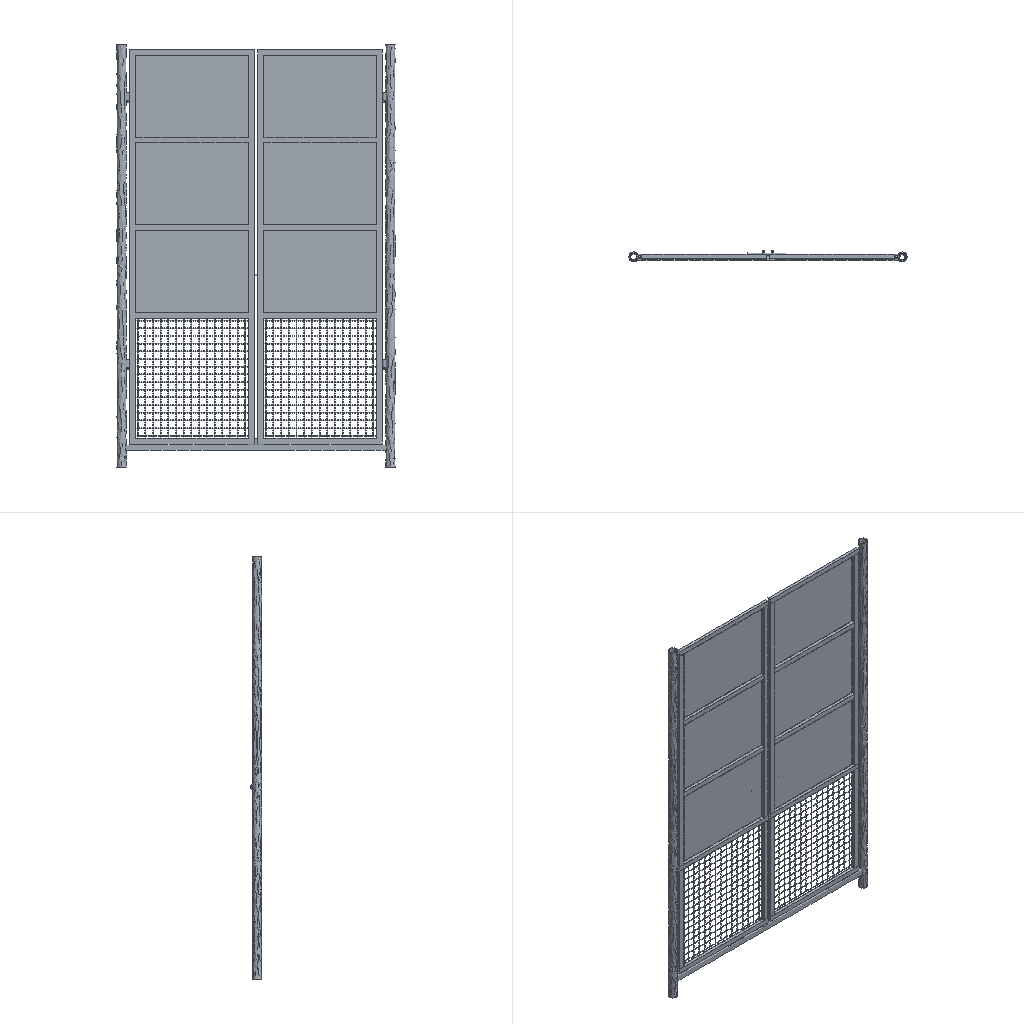Simulation study | ansys workbench
Set-up summary:
category,name,step,type,value,unit,region
solver,ansys_mapdl
solver,version,,,25.2
solver,version,,,25.2
solver,version,,,25.2
solver,version,,,25.2
solver,version,,,25.2
units,MKS,,stated
analysis,deck,,static,static
load_step,requested,,,1
analysis,nlgeom,,,True
mesh,nodes,,,121122
mesh,elements,,,99947
element_type,ANSYS 187 (type 1),,solid,19822
element_type,ANSYS 186 (type 2),,solid,561
element_type,ANSYS 187 (type 3),,solid,19785
element_type,ANSYS 187 (type 4),,solid,10615
element_type,ANSYS 174 (type 5),,contact,5385
element_type,ANSYS 170 (type 6),,target,5385
element_type,ANSYS 174 (type 7),,contact,6752
element_type,ANSYS 170 (type 8),,target,6752
element_type,ANSYS 174 (type 9),,contact,5458
element_type,ANSYS 170 (type 10),,target,5458
element_type,ANSYS 174 (type 11),,contact,6942
element_type,ANSYS 170 (type 12),,target,6942
element_type,ANSYS 154 (type 13),,surface,90
load,load commands in deck,,count,3
bc,support commands in deck,,count,1
named_set,_FIXEDSU,,component
material,1,,in results
material,2,,in results
material,3,,in results
material,1,,in results
material,3,,in results
material,1,,in results
material,1,,in results
material,4,,in results
material,1,,in results
material,2,,in results
material,3,,in results
material,4,,in results
check,setup vs results,,match,24537 contact/target element(s) of the setup are not in the results: solve.out records that the solver deleted 24537 by its trimming logic; 90 surface effect element(s) are not in the reader's mesh and were not compared
Ansys APDL input file, long lists of numbers shortened:
/batch
/config,noeldb,1     ! force off writing results to database
*get,_wallstrt,active,,time,wall
! ANSYS input file written by Workbench version 2025 R2
! File used for geometry attach: D:\å±é¨\fangan1\æ¹æ¡1_files\dp0\SYS\DM\SYS.dsco
/title,__1--____ (A5)
! ****** Begin Custom Load Command Snippet ******
/COM, ACT Extensions:
/COM,     LSDYNA, 2025.2
/COM,/COM,     ANSYSMotion, 2025.2
/COM,
! ****** End   Custom Load Command Snippet ******
/com,--- Data in consistent MKS units. See Solving Units in the help system for more information.
/units,MKS
/nopr
/wb,file,start              !  signify a WB generated input file
/prep7
! Turn off shape checking because checks already performed inside WB mesher.
! See help system for more information.
SHPP,OFF,,NOWARN
/nolist
etcon,set             ! allow ANSYS to choose best KEYOP's for 180x elements, resets any applicable keyopt to MAPDL defaults
/com,*********** Send User Defined Coordinate System(s) ***********
csys,0
/com,*********** Nodes for the whole assembly ***********
nblock,3,,133234
(1i9,3e20.9e3)
    48322     1.737721569E+00     1.701438756E-02    -1.199439081E+00
! (121121 more lines like these left out)
-1
/wb,elem,start            !  set before creation of elements
/com,*********** Elements for Body 1 'SYS\__' ***********
et,1,187
MAT,1 $ TYPE,1 $ REAL,1 $ SECNUM,1 $ ESYS,0
eblock,11,COMPACT,,19822
(11i9)
        1        1     8739     8742     8896     9317    47651     9318     9319    47655    47673
! (19821 more lines like these left out)
-1
secnum,1    ! reset the section ID to default
/com,*********** Elements for Body 2 'SYS\__' ***********
et,2,186
keyo,2,2,1          ! set full integration on SOLID186
MAT,2 $ TYPE,2 $ REAL,2 $ SECNUM,2 $ ESYS,0
eblock,11,COMPACT,,561
(11i9)
    19823    48322    48325    48329    48328    48729    48726    48722    48723    49155    49168
! (1121 more lines like these left out)
-1
secnum,1    ! reset the section ID to default
/com,*********** Elements for Body 3 'SYS\__' ***********
et,3,187
MAT,3 $ TYPE,3 $ REAL,3 $ SECNUM,3 $ ESYS,0
eblock,11,COMPACT,,19785
(11i9)
    20384    53935    60208    60034    53939    79578    98792    79576    79574    79599    79598
! (19784 more lines like these left out)
-1
secnum,1    ! reset the section ID to default
/com,*********** Elements for Body 4 'SYS\__' ***********
et,4,187
MAT,4 $ TYPE,4 $ REAL,4 $ SECNUM,4 $ ESYS,0
eblock,11,COMPACT,,10615
(11i9)
    40169    99585    99920    99586    99845   103304   103312   103298   103302   104804   103311
! (10614 more lines like these left out)
-1
secnum,1    ! reset the section ID to default
/wb,elem,end               !  done creating elements
toffst,273.15,      ! Temperature offset from absolute zero
/com,*********** Set Reference Temperature ***********
tref,22.
/wb,mat,start              !  starting to send materials
/com,*********** Send Materials ***********
Temperature = 'TEMP' ! Temperature
MP,DENS,1,7850,	! kg m^-3
MP,ALPX,1,1.2e-05,	! C^-1
MP,C,1,434,	! J kg^-1 C^-1
MP,KXX,1,60.5,	! W m^-1 C^-1
MP,RSVX,1,1.7e-07,	! kg m^3 A^-2 s^-3
MP,EX,1,200000000000,	! Pa
MP,NUXY,1,0.3,
MP,MURX,1,10000,
Temperature = 'TEMP' ! Temperature
MP,DENS,2,7850,	! kg m^-3
MP,ALPX,2,1.2e-05,	! C^-1
MP,C,2,434,	! J kg^-1 C^-1
MP,KXX,2,60.5,	! W m^-1 C^-1
MP,RSVX,2,1.7e-07,	! kg m^3 A^-2 s^-3
MP,EX,2,200000000000,	! Pa
MP,NUXY,2,0.3,
MP,MURX,2,10000,
Temperature = 'TEMP' ! Temperature
MP,DENS,3,7850,	! kg m^-3
MP,ALPX,3,1.2e-05,	! C^-1
MP,C,3,434,	! J kg^-1 C^-1
MP,KXX,3,60.5,	! W m^-1 C^-1
MP,RSVX,3,1.7e-07,	! kg m^3 A^-2 s^-3
MP,EX,3,200000000000,	! Pa
MP,NUXY,3,0.3,
MP,MURX,3,10000,
Temperature = 'TEMP' ! Temperature
MP,DENS,4,7850,	! kg m^-3
MP,ALPX,4,1.2e-05,	! C^-1
MP,C,4,434,	! J kg^-1 C^-1
MP,KXX,4,60.5,	! W m^-1 C^-1
MP,RSVX,4,1.7e-07,	! kg m^3 A^-2 s^-3
MP,EX,4,200000000000,	! Pa
MP,NUXY,4,0.3,
MP,MURX,4,10000,
/wb,mat,end                !  done sending materials
!************************* Model Summary ********************
!SYS\å®ä½,	ç»æé¢,	matid,	1
!SYS\å®ä½,	ç»æé¢,	matid,	2
!SYS\å®ä½,	ç»æé¢,	matid,	3
!SYS\å®ä½,	ç»æé¢,	matid,	4
!************************* End Model Summary ********************
! get the diagonal of the bounding box. Needed later for other things
*get,_xmin,node,,mnloc,x
*get,_ymin,node,,mnloc,y
*get,_zmin,node,,mnloc,z
*get,_xmax,node,,mxloc,x
*get,_ymax,node,,mxloc,y
*get,_zmax,node,,mxloc,z
_ASMDIAG=(_xmax-_xmin)*(_xmax-_xmin)+(_ymax-_ymin)*(_ymax-_ymin)+(_zmax-_zmin)*(_zmax-_zmin)
_ASMDIAG=SQRT(_ASMDIAG)
/wb,contact,start          !  starting to send contact
/com,*********** Create Contact "ÎÞÄ¦²Á - SYS\ÊµÌå Î»ÓÚ SYS\ÊµÌå" ***********
/com,            Real Constant Set For Above Contact Is 6 & 5
*set,tid,6
*set,cid,5
r,tid
r,cid
et,tid,170
et,cid,174
MAT,6 $ TYPE,6 $ REAL,6 $ SECNUM,6 $ ESYS,0
eblock,11,COMPACT,,4977
(11i9)
    96840      950      817     4528     4528    15468    15474     4528    16378
! (4976 more lines like these left out)
-1
secnum,1    ! reset the section ID to default
MAT,5 $ TYPE,5 $ REAL,5 $ SECNUM,5 $ ESYS,0
eblock,11,COMPACT,,4977
(11i9)
   101817      950      817     4528     4528    15468    15474     4528    16378
! (4976 more lines like these left out)
-1
secnum,1    ! reset the section ID to default
MAT,5 $ TYPE,5 $ REAL,6 $ SECNUM,5 $ ESYS,0
eblock,11,COMPACT,,408
(11i9)
   106794    49096    49097    49098    48746    51264    51266    50517    50516
! (407 more lines like these left out)
-1
secnum,1    ! reset the section ID to default
MAT,6 $ TYPE,6 $ REAL,5 $ SECNUM,6 $ ESYS,0
eblock,11,COMPACT,,408
(11i9)
   107202    49096    49097    49098    48746    51264    51266    50517    50516
! (407 more lines like these left out)
-1
secnum,1    ! reset the section ID to default
keyo,cid,8,2               ! auto create asymmetric contact (from Program Controlled setting)
keyo,cid,10,0              ! adjust contact stiffness each NR iteration (from Program Controlled setting)
keyo,cid,12,0              ! standard contact
keyo,cid,2,0               ! augmented Lagrange (from Program Controlled setting)
keyo,cid,4,0               ! on Gauss point (from Program Controlled setting)
keyo,cid,9,0               ! use real geometry with stepped effects
keyo,cid,7,0               ! No Prediction
rmod,tid,3,1.       ! FKN
rmod,tid,5,0.       ! ICONT
rmod,tid,6,0.       ! PINB
rmod,tid,10,0.      ! CNOF
rmod,tid,12,0.      ! FKT
rmod,tid,36,35      ! WB DSID
rmod,cid,3,1.       ! FKN
rmod,cid,5,0.       ! ICONT
rmod,cid,6,0.       ! PINB
rmod,cid,10,0.      ! CNOF
rmod,cid,12,0.      ! FKT
rmod,cid,36,35      ! WB DSID
/com,*********** Create Contact "ÎÞ·ÖÀë - SYS\ÊµÌå Î»ÓÚ SYS\ÊµÌå" ***********
/com,            Real Constant Set For Above Contact Is 8 & 7
*set,tid,8
*set,cid,7
r,tid
r,cid
et,tid,170
et,cid,174
MAT,8 $ TYPE,8 $ REAL,8 $ SECNUM,8 $ ESYS,0
eblock,11,COMPACT,,5292
(11i9)
   107610     2364     8805     8814     8814    26129    47859     8814    26131
! (5291 more lines like these left out)
-1
secnum,1    ! reset the section ID to default
MAT,7 $ TYPE,7 $ REAL,7 $ SECNUM,7 $ ESYS,0
eblock,11,COMPACT,,5292
(11i9)
   112902     2364     8805     8814     8814    26129    47859     8814    26131
! (5291 more lines like these left out)
-1
secnum,1    ! reset the section ID to default
MAT,7 $ TYPE,7 $ REAL,8 $ SECNUM,7 $ ESYS,0
eblock,11,COMPACT,,1460
(11i9)
   118194    99804    99806    99805    99805   104676   104680    99805   104675
! (1459 more lines like these left out)
-1
secnum,1    ! reset the section ID to default
MAT,8 $ TYPE,8 $ REAL,7 $ SECNUM,8 $ ESYS,0
eblock,11,COMPACT,,1460
(11i9)
   119654    99804    99806    99805    99805   104676   104680    99805   104675
! (1459 more lines like these left out)
-1
secnum,1    ! reset the section ID to default
keyo,cid,8,2               ! auto create asymmetric contact (from Program Controlled setting)
keyo,cid,10,0              ! adjust contact stiffness each NR iteration (from Program Controlled setting)
keyo,cid,12,4              ! no separation always
keyo,cid,2,0               ! augmented Lagrange (from Program Controlled setting)
keyo,cid,4,0               ! on Gauss point (from Program Controlled setting)
keyo,cid,9,1               ! ignore initial gaps/penetration
keyo,cid,7,0               ! No Prediction
rmod,tid,3,1.       ! FKN
rmod,tid,5,0.       ! ICONT
rmod,tid,6,0.       ! PINB
rmod,tid,10,0.      ! CNOF
rmod,tid,12,0.      ! FKT
rmod,tid,36,38      ! WB DSID
rmod,cid,3,1.       ! FKN
rmod,cid,5,0.       ! ICONT
rmod,cid,6,0.       ! PINB
rmod,cid,10,0.      ! CNOF
rmod,cid,12,0.      ! FKT
rmod,cid,36,38      ! WB DSID
/com,*********** Create Contact "ÎÞ·ÖÀë - SYS\ÊµÌå Î»ÓÚ SYS\ÊµÌå" ***********
/com,            Real Constant Set For Above Contact Is 10 & 9
*set,tid,10
*set,cid,9
r,tid
r,cid
et,tid,170
et,cid,174
MAT,10 $ TYPE,10 $ REAL,10 $ SECNUM,10 $ ESYS,0
eblock,11,COMPACT,,408
(11i9)
   121114    49096    49097    49098    48746    51264    51266    50517    50516
! (407 more lines like these left out)
-1
secnum,1    ! reset the section ID to default
MAT,9 $ TYPE,9 $ REAL,9 $ SECNUM,9 $ ESYS,0
eblock,11,COMPACT,,408
(11i9)
   121522    49096    49097    49098    48746    51264    51266    50517    50516
! (407 more lines like these left out)
-1
secnum,1    ! reset the section ID to default
MAT,9 $ TYPE,9 $ REAL,10 $ SECNUM,9 $ ESYS,0
eblock,11,COMPACT,,5050
(11i9)
   121930    55716    51961    52095    52095    65089    65084    52095    66016
! (5049 more lines like these left out)
-1
secnum,1    ! reset the section ID to default
MAT,10 $ TYPE,10 $ REAL,9 $ SECNUM,10 $ ESYS,0
eblock,11,COMPACT,,5050
(11i9)
   126980    55716    51961    52095    52095    65089    65084    52095    66016
! (5049 more lines like these left out)
-1
secnum,1    ! reset the section ID to default
keyo,cid,8,2               ! auto create asymmetric contact (from Program Controlled setting)
keyo,cid,10,0              ! adjust contact stiffness each NR iteration (from Program Controlled setting)
keyo,cid,12,4              ! no separation always
keyo,cid,2,0               ! augmented Lagrange (from Program Controlled setting)
keyo,cid,4,0               ! on Gauss point (from Program Controlled setting)
keyo,cid,9,1               ! ignore initial gaps/penetration
keyo,cid,7,0               ! No Prediction
rmod,tid,3,1.       ! FKN
rmod,tid,5,0.       ! ICONT
rmod,tid,6,0.       ! PINB
rmod,tid,10,0.      ! CNOF
rmod,tid,12,0.      ! FKT
rmod,tid,36,41      ! WB DSID
rmod,cid,3,1.       ! FKN
rmod,cid,5,0.       ! ICONT
rmod,cid,6,0.       ! PINB
rmod,cid,10,0.      ! CNOF
rmod,cid,12,0.      ! FKT
rmod,cid,36,41      ! WB DSID
/com,*********** Create Contact "ÎÞÄ¦²Á - SYS\ÊµÌå Î»ÓÚ SYS\ÊµÌå" ***********
/com,            Real Constant Set For Above Contact Is 12 & 11
*set,tid,12
*set,cid,11
r,tid
r,cid
et,tid,170
et,cid,174
MAT,12 $ TYPE,12 $ REAL,12 $ SECNUM,12 $ ESYS,0
eblock,11,COMPACT,,5274
(11i9)
   132030    53953    53956    53946    53946    79669    79631    53946    79630
! (5273 more lines like these left out)
-1
secnum,1    ! reset the section ID to default
MAT,11 $ TYPE,11 $ REAL,11 $ SECNUM,11 $ ESYS,0
eblock,11,COMPACT,,5274
(11i9)
   137304    53953    53956    53946    53946    79669    79631    53946    79630
! (5273 more lines like these left out)
-1
secnum,1    ! reset the section ID to default
MAT,11 $ TYPE,11 $ REAL,12 $ SECNUM,11 $ ESYS,0
eblock,11,COMPACT,,1668
(11i9)
   142578    99804    99806    99805    99805   104676   104680    99805   104675
! (1667 more lines like these left out)
-1
secnum,1    ! reset the section ID to default
MAT,12 $ TYPE,12 $ REAL,11 $ SECNUM,12 $ ESYS,0
eblock,11,COMPACT,,1668
(11i9)
   144246    99804    99806    99805    99805   104676   104680    99805   104675
! (1667 more lines like these left out)
-1
secnum,1    ! reset the section ID to default
keyo,cid,8,2               ! auto create asymmetric contact (from Program Controlled setting)
keyo,cid,10,0              ! adjust contact stiffness each NR iteration (from Program Controlled setting)
keyo,cid,12,0              ! standard contact
keyo,cid,2,0               ! augmented Lagrange (from Program Controlled setting)
keyo,cid,4,0               ! on Gauss point (from Program Controlled setting)
keyo,cid,9,0               ! use real geometry with stepped effects
keyo,cid,7,0               ! No Prediction
rmod,tid,3,1.       ! FKN
rmod,tid,5,0.       ! ICONT
rmod,tid,6,0.       ! PINB
rmod,tid,10,0.      ! CNOF
rmod,tid,12,0.      ! FKT
rmod,tid,36,44      ! WB DSID
rmod,cid,3,1.       ! FKN
rmod,cid,5,0.       ! ICONT
rmod,cid,6,0.       ! PINB
rmod,cid,10,0.      ! CNOF
rmod,cid,12,0.      ! FKT
rmod,cid,36,44      ! WB DSID
nsel,all
esel,all
/wb,contact,end            !  done creating contacts
/golist
/wb,load,start             !  starting to send loads
/com,*********** Fixed Supports ***********
CMBLOCK,_FIXEDSU,NODE,      192
(8i10)
     99609    -99624     99661    -99676     99684    -99697     99718    -99731
! (23 more lines like these left out)
cmsel,s,_FIXEDSU
d,all,all
nsel,all
/com,*********** Define Force Using Surface Effect Elements ***********
local,12,0,0.,0.,0.,0.,0.,0.
csys,0
et,13,154
MAT,13 $ TYPE,13 $ REAL,13 $ SECNUM,13 $ ESYS,12
eblock,11,COMPACT,,90
(11i9)
   145914     9156     8762     9166     9166    47748    47749     9166    48281
! (89 more lines like these left out)
-1
secnum,1    ! reset the section ID to default
esel,s,type,,13
keyop,13,2,1        ! Apply load in local coordinate system
keyop,13,7,1        ! Use original area so load is constant in large deformation
esel,all
/gst,on,on
fini
*get,_numnode,node,0,count
*get,_numelem,elem,0,count
*get, _MAXELEMNUM, elem, 0, NUM, MAX
*get, _MAXNODENUM, node, 0, NUM, MAX
*get, _MAXELEMTYPE, etyp, 0, NUM, MAX
*get, _MAXREALCONST, rcon, 0, NUM, MAX
/go
/wb,load,end               !  done creating loads
/com,--- Number of total nodes = %_numnode%
/com,--- Number of contact elements = 49164
/com,--- Number of spring elements = 0
/com,--- Number of bearing elements = 0
/com,--- Number of solid elements = 50783
/com,--- Number of condensed parts = 0
/com,--- Number of total elements = %_numelem%
*get,_wallbsol,active,,time,wall
/com,****************************************************************************
/com,*************************    SOLUTION       ********************************
/com,****************************************************************************
/solu
antype,0                   ! static analysis
nlgeom,on                  ! Turn on Large Deformation Effects
_thickRatio=0.25    ! Ratio of thick parts in the model
eqsl,sparse,,,,,1
cntr,print,1               ! print out contact info and also make no initial contact an error
cncheck,dmp		!	Enable program controlled contact splitting for distributed memory parallel run
dmpoption,emat,no             ! Don't combine emat file for DANSYS
dmpoption,esav,no             ! Don't combine esav file for DANSYS
nldiag,cont,iter           ! print out contact info each equilibrium iteration
rescontrol,define,last,last,,dele	   ! Program Controlled
/com,****************************************************
/com,******************* SOLVE FOR LS 1 OF 1 ****************
esel,s,type,,13
nsle
sfe,all,1,pres,1,0.
sfe,all,2,pres,1,2376.049
sfe,all,3,pres,1,6.71851560076343e-012
nsel,all
esel,all
/nopr
/gopr
autots,on                  ! Workbench Program Controlled automatic time stepping
nsub,1,10,1                ! due to presence of general nonlinear
time,1.
outres,erase
outres,all,none
outres,nsol,all,
outres,rsol,all
outres,eangl,all
outres,etmp,all
outres,veng,all
outres,strs,all,
outres,epel,all,
outres,eppl,all,
outres,cont,all,
! *********** WB SOLVE COMMAND ***********
! check interactive state
*get,ANSINTER_,active,,int
*if,ANSINTER_,ne,0,then
/eof
*endif
solve
/com *************** Write FE CONNECTORS *********
CEWRITE,file,ce,,INTE
/com,****************************************************
/com,*************** FINISHED SOLVE FOR LS 1 *************
*get,_wallasol,active,,time,wall
/nopr
*get,_numnode,node,0,count
*get,_numelem,elem,0,count
*get, _MAXELEMNUM, elem, 0, NUM, MAX
*get, _MAXNODENUM, node, 0, NUM, MAX,,,INTERNAL
*get, _MAXELEMTYPE, etyp, 0, NUM, MAX
*get, _MAXREALCONST, rcon, 0, NUM, MAX
*get,_NSOLTHREADS,active,0,ntfs
*get,_NSOLPROCESSES,active,0,npfs
/gopr
/post1
xmlo,ENCODING,ISO-8859-1
xmlo,parm
/xml,parm,xml
fini
/gopr
*get,_walldone,active,,time,wall
_preptime=(_wallbsol-_wallstrt)*3600
_solvtime=(_wallasol-_wallbsol)*3600
_posttime=(_walldone-_wallasol)*3600
_totaltim=(_walldone-_wallstrt)*3600
*get,_dlbratio,active,0,solu,dlbr
*get,_combtime,active,0,solu,comb
*get,_ssmode,active,0,solu,ssmm
*get,_ndofs,active,0,solu,ndof
*get,_sol_end_time,active,0,set,time
*if,_sol_end_time,eq,1.,then
/fclean				!clean distributed files
*endif
/com,--- Total number of nodes = %_numnode%
/com,--- Total number of elements = %_numelem%
/com,--- Element load balance ratio = %_dlbratio%
/com,--- Time to combine distributed files = %_combtime%
/com,--- Sparse memory mode = %_ssmode%
/com,--- Number of DOF = %_ndofs%
/wb,file,end               ! done with WB generated input
Results summary:
result,analysis,,,static
result,last_loadstep,,,1
result,primary field,,,displacement
result,mass,,,13.838,"MKS: m, kg, N, s, V, A, degC"
result,analysis,,,static
result,last_loadstep,,,1
result,primary field,,,displacement
result,reaction total,1,FX,0.0,N
result,reaction total,1,FY,0.0,N
result,reaction total,1,FZ,0.0,N
result,mass,,,13.696,"MKS: m, kg, N, s, V, A, degC"
result,analysis,,,static
result,last_loadstep,,,1
result,primary field,,,displacement
result,reaction total,1,FX,0.0,N
result,reaction total,1,FY,0.0,N
result,reaction total,1,FZ,0.0,N
result,mass,,,3.829,"MKS: m, kg, N, s, V, A, degC"
result,analysis,,,static
result,last_loadstep,,,1
result,primary field,,,displacement
result,reaction total,1,FX,0.002628,N
result,reaction total,1,FY,-60,N
result,reaction total,1,FZ,-0.02645,N
result,mass,,,28.851,"MKS: m, kg, N, s, V, A, degC"
result,analysis,,,static
result,last_loadstep,,,1
result,primary field,,,displacement
result,reaction total,1,FX,0.002628,N
result,reaction total,1,FY,-60,N
result,reaction total,1,FZ,-0.02645,N
result,mass,,,60.214,"MKS: m, kg, N, s, V, A, degC"